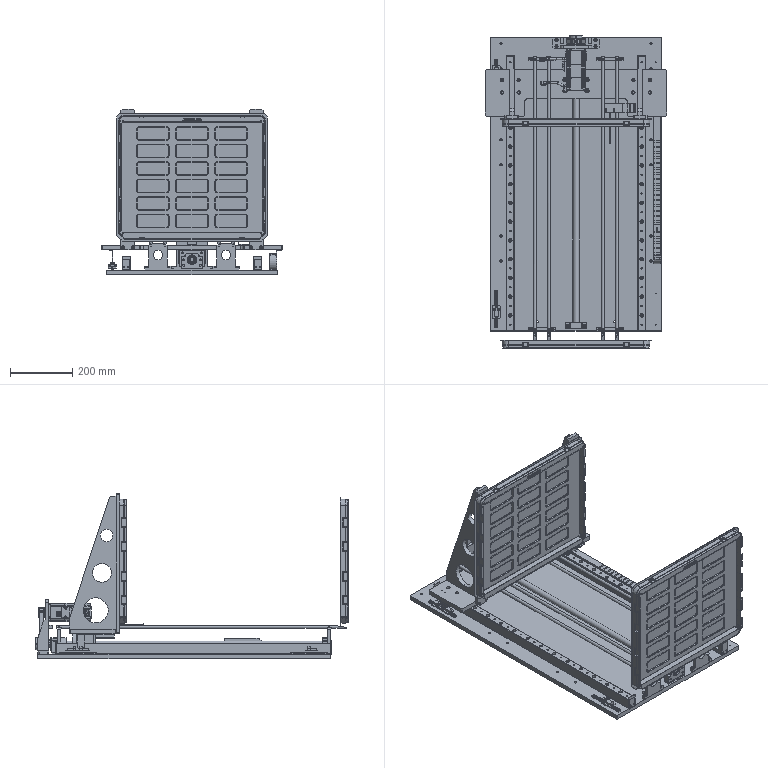Part | NX | 58 solids | 4791 faces | volume 23724474 mm3 | plane 2681 | cylinder 1617 | spline 266 | cone 225 | torus 2 | commonest cylinder face diameters 10 x170 13 x144 3 x130 5 x108 4.2 x102 4 x91